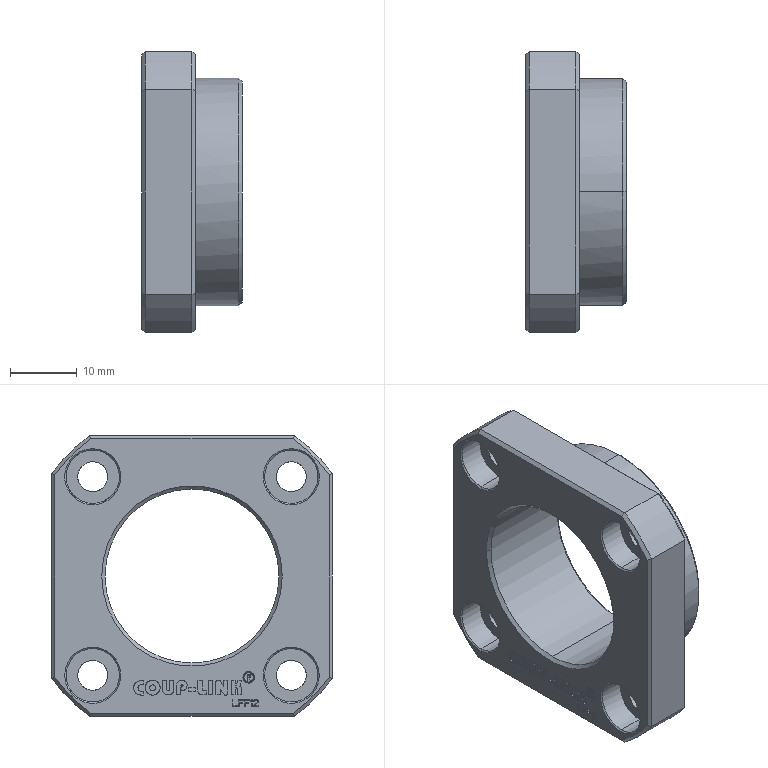Part | STEP file | LFF12-1-1 | 1 solid | 683 faces | box 15 x 42 x 42 mm | volume 10904 mm3 | plane 629 | cone 30 | cylinder 24 | commonest cylinder face diameters 4.5 x8 8 x8 52 x4 26 x2 34 x2